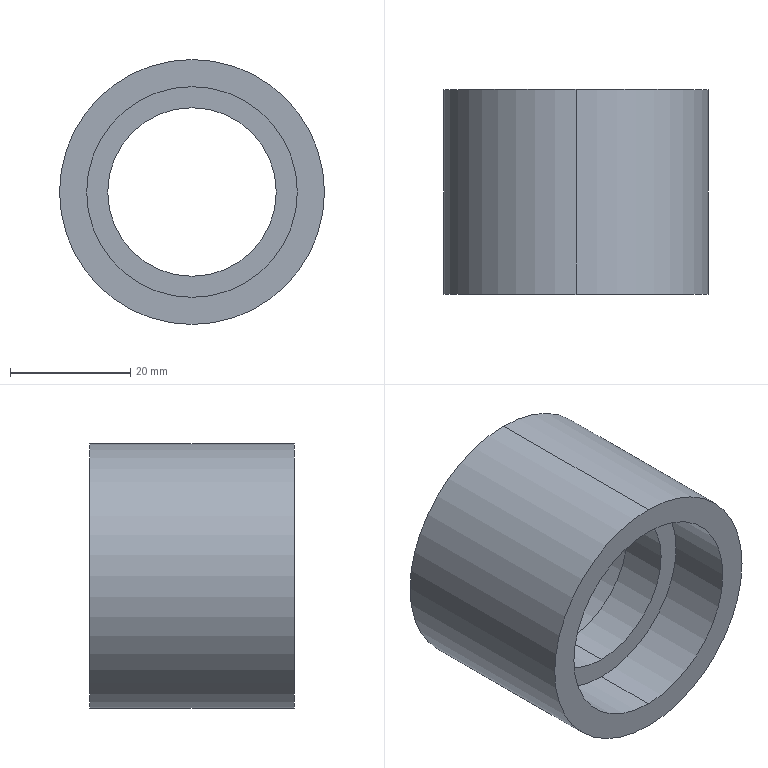Part | SolidWorks | features BaseBody 1 | 1 solid | 12 faces | box 44 x 34 x 44 mm | volume 21757 mm3 | cylinder 8 | plane 4 | commonest cylinder face diameters 35 x4 28 x2 44 x2
STEP:
#1=CARTESIAN_POINT('',(0.,17.,-22.));
#2=VERTEX_POINT('',#1);
#3=CARTESIAN_POINT('',(0.,17.,22.));
#4=VERTEX_POINT('',#3);
#5=CARTESIAN_POINT('',(0.,17.,0.));
#6=DIRECTION('',(0.,-1.,0.));
#7=DIRECTION('',(0.,0.,-1.));
#8=AXIS2_PLACEMENT_3D('',#5,#6,#7);
#9=CIRCLE('',#8,22.);
#10=EDGE_CURVE('',#2,#4,#9,.T.);
#11=ORIENTED_EDGE('',*,*,#10,.T.);
#12=CARTESIAN_POINT('',(0.,-17.,22.));
#13=VERTEX_POINT('',#12);
#14=CARTESIAN_POINT('',(0.,17.,22.));
#15=DIRECTION('',(0.,-1.,0.));
#16=VECTOR('',#15,1000.);
#17=LINE('',#14,#16);
#18=EDGE_CURVE('',#4,#13,#17,.T.);
#19=ORIENTED_EDGE('',*,*,#18,.T.);
#20=CARTESIAN_POINT('',(0.,-17.,-22.));
#21=VERTEX_POINT('',#20);
#22=CARTESIAN_POINT('',(0.,-17.,0.));
#23=DIRECTION('',(0.,1.,0.));
#24=DIRECTION('',(0.,0.,-1.));
#25=AXIS2_PLACEMENT_3D('',#22,#23,#24);
#26=CIRCLE('',#25,22.);
#27=EDGE_CURVE('',#13,#21,#26,.T.);
#28=ORIENTED_EDGE('',*,*,#27,.T.);
#29=CARTESIAN_POINT('',(0.,17.,-22.));
#30=DIRECTION('',(0.,-1.,0.));
#31=VECTOR('',#30,1000.);
#32=LINE('',#29,#31);
#33=EDGE_CURVE('',#2,#21,#32,.T.);
#34=ORIENTED_EDGE('',*,*,#33,.F.);
#35=EDGE_LOOP('',(#11,#19,#28,#34));
#36=FACE_OUTER_BOUND('',#35,.T.);
#37=CARTESIAN_POINT('',(0.,17.,0.));
#38=DIRECTION('',(0.,-1.,0.));
#39=DIRECTION('',(0.,0.,-1.));
#40=AXIS2_PLACEMENT_3D('',#37,#38,#39);
#41=CYLINDRICAL_SURFACE('',#40,22.);
#42=ADVANCED_FACE('',(#36),#41,.T.);
#43=CARTESIAN_POINT('',(0.,-6.,17.5));
#44=VERTEX_POINT('',#43);
#45=CARTESIAN_POINT('',(0.,-6.,-17.5));
#46=VERTEX_POINT('',#45);
#47=CARTESIAN_POINT('',(0.,-6.,0.));
#48=DIRECTION('',(0.,-1.,0.));
#49=DIRECTION('',(0.,0.,-1.));
#50=AXIS2_PLACEMENT_3D('',#47,#48,#49);
#51=CIRCLE('',#50,17.5);
#52=EDGE_CURVE('',#44,#46,#51,.T.);
#53=ORIENTED_EDGE('',*,*,#52,.F.);
#54=CARTESIAN_POINT('',(0.,-17.,17.5));
#55=VERTEX_POINT('',#54);
#56=CARTESIAN_POINT('',(0.,-6.,17.5));
#57=DIRECTION('',(0.,-1.,0.));
#58=VECTOR('',#57,1000.);
#59=LINE('',#56,#58);
#60=EDGE_CURVE('',#44,#55,#59,.T.);
#61=ORIENTED_EDGE('',*,*,#60,.T.);
#62=CARTESIAN_POINT('',(0.,-17.,-17.5));
#63=VERTEX_POINT('',#62);
#64=CARTESIAN_POINT('',(0.,-17.,0.));
#65=DIRECTION('',(0.,-1.,0.));
#66=DIRECTION('',(0.,0.,-1.));
#67=AXIS2_PLACEMENT_3D('',#64,#65,#66);
#68=CIRCLE('',#67,17.5);
#69=EDGE_CURVE('',#55,#63,#68,.T.);
#70=ORIENTED_EDGE('',*,*,#69,.T.);
#71=CARTESIAN_POINT('',(0.,-6.,-17.5));
#72=DIRECTION('',(0.,-1.,0.));
#73=VECTOR('',#72,1000.);
#74=LINE('',#71,#73);
#75=EDGE_CURVE('',#46,#63,#74,.T.);
#76=ORIENTED_EDGE('',*,*,#75,.F.);
#77=EDGE_LOOP('',(#53,#61,#70,#76));
#78=FACE_OUTER_BOUND('',#77,.T.);
#79=CARTESIAN_POINT('',(0.,-6.,0.));
#80=DIRECTION('',(0.,-1.,0.));
#81=DIRECTION('',(0.,0.,-1.));
#82=AXIS2_PLACEMENT_3D('',#79,#80,#81);
#83=CYLINDRICAL_SURFACE('',#82,17.5);
#84=ADVANCED_FACE('',(#78),#83,.F.);
#85=CARTESIAN_POINT('',(0.,2.,-17.5));
#86=VERTEX_POINT('',#85);
#87=CARTESIAN_POINT('',(0.,2.,17.5));
#88=VERTEX_POINT('',#87);
#89=CARTESIAN_POINT('',(0.,2.,0.));
#90=DIRECTION('',(0.,1.,0.));
#91=DIRECTION('',(0.,0.,1.));
#92=AXIS2_PLACEMENT_3D('',#89,#90,#91);
#93=CIRCLE('',#92,17.5);
#94=EDGE_CURVE('',#86,#88,#93,.T.);
#95=ORIENTED_EDGE('',*,*,#94,.F.);
#96=CARTESIAN_POINT('',(0.,17.,-17.5));
#97=VERTEX_POINT('',#96);
#98=CARTESIAN_POINT('',(0.,2.,-17.5));
#99=DIRECTION('',(0.,1.,0.));
#100=VECTOR('',#99,1000.);
#101=LINE('',#98,#100);
#102=EDGE_CURVE('',#86,#97,#101,.T.);
#103=ORIENTED_EDGE('',*,*,#102,.T.);
#104=CARTESIAN_POINT('',(0.,17.,17.5));
#105=VERTEX_POINT('',#104);
#106=CARTESIAN_POINT('',(0.,17.,0.));
#107=DIRECTION('',(0.,-1.,0.));
#108=DIRECTION('',(0.,0.,1.));
#109=AXIS2_PLACEMENT_3D('',#106,#107,#108);
#110=CIRCLE('',#109,17.5);
#111=EDGE_CURVE('',#105,#97,#110,.T.);
#112=ORIENTED_EDGE('',*,*,#111,.F.);
#113=CARTESIAN_POINT('',(0.,2.,17.5));
#114=DIRECTION('',(0.,1.,0.));
#115=VECTOR('',#114,1000.);
#116=LINE('',#113,#115);
#117=EDGE_CURVE('',#88,#105,#116,.T.);
#118=ORIENTED_EDGE('',*,*,#117,.F.);
#119=EDGE_LOOP('',(#95,#103,#112,#118));
#120=FACE_OUTER_BOUND('',#119,.T.);
#121=CARTESIAN_POINT('',(0.,2.,0.));
#122=DIRECTION('',(0.,1.,0.));
#123=DIRECTION('',(0.,0.,1.));
#124=AXIS2_PLACEMENT_3D('',#121,#122,#123);
#125=CYLINDRICAL_SURFACE('',#124,17.5);
#126=ADVANCED_FACE('',(#120),#125,.F.);
#127=CARTESIAN_POINT('',(0.,-6.,-14.));
#128=VERTEX_POINT('',#127);
#129=CARTESIAN_POINT('',(0.,-6.,14.));
#130=VERTEX_POINT('',#129);
#131=CARTESIAN_POINT('',(0.,-6.,0.));
#132=DIRECTION('',(0.,1.,0.));
#133=DIRECTION('',(0.,0.,1.));
#134=AXIS2_PLACEMENT_3D('',#131,#132,#133);
#135=CIRCLE('',#134,14.);
#136=EDGE_CURVE('',#128,#130,#135,.T.);
#137=ORIENTED_EDGE('',*,*,#136,.F.);
#138=CARTESIAN_POINT('',(0.,2.,-14.));
#139=VERTEX_POINT('',#138);
#140=CARTESIAN_POINT('',(0.,-17.,-14.));
#141=DIRECTION('',(0.,1.,0.));
#142=VECTOR('',#141,1000.);
#143=LINE('',#140,#142);
#144=EDGE_CURVE('',#128,#139,#143,.T.);
#145=ORIENTED_EDGE('',*,*,#144,.T.);
#146=CARTESIAN_POINT('',(0.,2.,14.));
#147=VERTEX_POINT('',#146);
#148=CARTESIAN_POINT('',(0.,2.,0.));
#149=DIRECTION('',(0.,-1.,0.));
#150=DIRECTION('',(0.,0.,1.));
#151=AXIS2_PLACEMENT_3D('',#148,#149,#150);
#152=CIRCLE('',#151,14.);
#153=EDGE_CURVE('',#147,#139,#152,.T.);
#154=ORIENTED_EDGE('',*,*,#153,.F.);
#155=CARTESIAN_POINT('',(0.,-17.,14.));
#156=DIRECTION('',(0.,1.,0.));
#157=VECTOR('',#156,1000.);
#158=LINE('',#155,#157);
#159=EDGE_CURVE('',#130,#147,#158,.T.);
#160=ORIENTED_EDGE('',*,*,#159,.F.);
#161=EDGE_LOOP('',(#137,#145,#154,#160));
#162=FACE_OUTER_BOUND('',#161,.T.);
#163=CARTESIAN_POINT('',(0.,-17.,0.));
#164=DIRECTION('',(0.,1.,0.));
#165=DIRECTION('',(0.,0.,1.));
#166=AXIS2_PLACEMENT_3D('',#163,#164,#165);
#167=CYLINDRICAL_SURFACE('',#166,14.);
#168=ADVANCED_FACE('',(#162),#167,.F.);
#169=ORIENTED_EDGE('',*,*,#18,.F.);
#170=CARTESIAN_POINT('',(0.,17.,0.));
#171=DIRECTION('',(0.,-1.,0.));
#172=DIRECTION('',(0.,0.,-1.));
#173=AXIS2_PLACEMENT_3D('',#170,#171,#172);
#174=CIRCLE('',#173,22.);
#175=EDGE_CURVE('',#4,#2,#174,.T.);
#176=ORIENTED_EDGE('',*,*,#175,.T.);
#177=ORIENTED_EDGE('',*,*,#33,.T.);
#178=CARTESIAN_POINT('',(0.,-17.,0.));
#179=DIRECTION('',(0.,1.,0.));
#180=DIRECTION('',(0.,0.,-1.));
#181=AXIS2_PLACEMENT_3D('',#178,#179,#180);
#182=CIRCLE('',#181,22.);
#183=EDGE_CURVE('',#21,#13,#182,.T.);
#184=ORIENTED_EDGE('',*,*,#183,.T.);
#185=EDGE_LOOP('',(#169,#176,#177,#184));
#186=FACE_OUTER_BOUND('',#185,.T.);
#187=CARTESIAN_POINT('',(0.,17.,0.));
#188=DIRECTION('',(0.,-1.,0.));
#189=DIRECTION('',(0.,0.,-1.));
#190=AXIS2_PLACEMENT_3D('',#187,#188,#189);
#191=CYLINDRICAL_SURFACE('',#190,22.);
#192=ADVANCED_FACE('',(#186),#191,.T.);
#193=ORIENTED_EDGE('',*,*,#183,.F.);
#194=ORIENTED_EDGE('',*,*,#27,.F.);
#195=EDGE_LOOP('',(#193,#194));
#196=FACE_OUTER_BOUND('',#195,.T.);
#197=CARTESIAN_POINT('',(0.,-17.,0.));
#198=DIRECTION('',(0.,-1.,0.));
#199=DIRECTION('',(0.,0.,-1.));
#200=AXIS2_PLACEMENT_3D('',#197,#198,#199);
#201=CIRCLE('',#200,17.5);
#202=EDGE_CURVE('',#63,#55,#201,.T.);
#203=ORIENTED_EDGE('',*,*,#202,.F.);
#204=ORIENTED_EDGE('',*,*,#69,.F.);
#205=EDGE_LOOP('',(#203,#204));
#206=FACE_BOUND('',#205,.T.);
#207=CARTESIAN_POINT('',(0.,-17.,0.));
#208=DIRECTION('',(0.,1.,0.));
#209=DIRECTION('',(0.,0.,1.));
#210=AXIS2_PLACEMENT_3D('',#207,#208,#209);
#211=PLANE('',#210);
#212=ADVANCED_FACE('',(#196,#206),#211,.F.);
#213=ORIENTED_EDGE('',*,*,#10,.F.);
#214=ORIENTED_EDGE('',*,*,#175,.F.);
#215=EDGE_LOOP('',(#213,#214));
#216=FACE_OUTER_BOUND('',#215,.T.);
#217=ORIENTED_EDGE('',*,*,#111,.T.);
#218=CARTESIAN_POINT('',(0.,17.,0.));
#219=DIRECTION('',(0.,-1.,0.));
#220=DIRECTION('',(0.,0.,1.));
#221=AXIS2_PLACEMENT_3D('',#218,#219,#220);
#222=CIRCLE('',#221,17.5);
#223=EDGE_CURVE('',#97,#105,#222,.T.);
#224=ORIENTED_EDGE('',*,*,#223,.T.);
#225=EDGE_LOOP('',(#217,#224));
#226=FACE_BOUND('',#225,.T.);
#227=CARTESIAN_POINT('',(0.,17.,0.));
#228=DIRECTION('',(0.,1.,0.));
#229=DIRECTION('',(0.,0.,1.));
#230=AXIS2_PLACEMENT_3D('',#227,#228,#229);
#231=PLANE('',#230);
#232=ADVANCED_FACE('',(#216,#226),#231,.T.);
#233=ORIENTED_EDGE('',*,*,#60,.F.);
#234=CARTESIAN_POINT('',(0.,-6.,0.));
#235=DIRECTION('',(0.,-1.,0.));
#236=DIRECTION('',(0.,0.,-1.));
#237=AXIS2_PLACEMENT_3D('',#234,#235,#236);
#238=CIRCLE('',#237,17.5);
#239=EDGE_CURVE('',#46,#44,#238,.T.);
#240=ORIENTED_EDGE('',*,*,#239,.F.);
#241=ORIENTED_EDGE('',*,*,#75,.T.);
#242=ORIENTED_EDGE('',*,*,#202,.T.);
#243=EDGE_LOOP('',(#233,#240,#241,#242));
#244=FACE_OUTER_BOUND('',#243,.T.);
#245=CARTESIAN_POINT('',(0.,-6.,0.));
#246=DIRECTION('',(0.,-1.,0.));
#247=DIRECTION('',(0.,0.,-1.));
#248=AXIS2_PLACEMENT_3D('',#245,#246,#247);
#249=CYLINDRICAL_SURFACE('',#248,17.5);
#250=ADVANCED_FACE('',(#244),#249,.F.);
#251=ORIENTED_EDGE('',*,*,#102,.F.);
#252=CARTESIAN_POINT('',(0.,2.,0.));
#253=DIRECTION('',(0.,1.,0.));
#254=DIRECTION('',(0.,0.,1.));
#255=AXIS2_PLACEMENT_3D('',#252,#253,#254);
#256=CIRCLE('',#255,17.5);
#257=EDGE_CURVE('',#88,#86,#256,.T.);
#258=ORIENTED_EDGE('',*,*,#257,.F.);
#259=ORIENTED_EDGE('',*,*,#117,.T.);
#260=ORIENTED_EDGE('',*,*,#223,.F.);
#261=EDGE_LOOP('',(#251,#258,#259,#260));
#262=FACE_OUTER_BOUND('',#261,.T.);
#263=CARTESIAN_POINT('',(0.,2.,0.));
#264=DIRECTION('',(0.,1.,0.));
#265=DIRECTION('',(0.,0.,1.));
#266=AXIS2_PLACEMENT_3D('',#263,#264,#265);
#267=CYLINDRICAL_SURFACE('',#266,17.5);
#268=ADVANCED_FACE('',(#262),#267,.F.);
#269=CARTESIAN_POINT('',(0.,-6.,0.));
#270=DIRECTION('',(0.,1.,0.));
#271=DIRECTION('',(0.,0.,1.));
#272=AXIS2_PLACEMENT_3D('',#269,#270,#271);
#273=CIRCLE('',#272,14.);
#274=EDGE_CURVE('',#130,#128,#273,.T.);
#275=ORIENTED_EDGE('',*,*,#274,.T.);
#276=ORIENTED_EDGE('',*,*,#136,.T.);
#277=EDGE_LOOP('',(#275,#276));
#278=FACE_BOUND('',#277,.T.);
#279=ORIENTED_EDGE('',*,*,#239,.T.);
#280=ORIENTED_EDGE('',*,*,#52,.T.);
#281=EDGE_LOOP('',(#279,#280));
#282=FACE_OUTER_BOUND('',#281,.T.);
#283=CARTESIAN_POINT('',(0.,-6.,0.));
#284=DIRECTION('',(0.,-1.,0.));
#285=DIRECTION('',(0.,0.,-1.));
#286=AXIS2_PLACEMENT_3D('',#283,#284,#285);
#287=PLANE('',#286);
#288=ADVANCED_FACE('',(#278,#282),#287,.T.);
#289=ORIENTED_EDGE('',*,*,#257,.T.);
#290=ORIENTED_EDGE('',*,*,#94,.T.);
#291=EDGE_LOOP('',(#289,#290));
#292=FACE_OUTER_BOUND('',#291,.T.);
#293=ORIENTED_EDGE('',*,*,#153,.T.);
#294=CARTESIAN_POINT('',(0.,2.,0.));
#295=DIRECTION('',(0.,-1.,0.));
#296=DIRECTION('',(0.,0.,1.));
#297=AXIS2_PLACEMENT_3D('',#294,#295,#296);
#298=CIRCLE('',#297,14.);
#299=EDGE_CURVE('',#139,#147,#298,.T.);
#300=ORIENTED_EDGE('',*,*,#299,.T.);
#301=EDGE_LOOP('',(#293,#300));
#302=FACE_BOUND('',#301,.T.);
#303=CARTESIAN_POINT('',(0.,2.,0.));
#304=DIRECTION('',(0.,1.,0.));
#305=DIRECTION('',(0.,0.,1.));
#306=AXIS2_PLACEMENT_3D('',#303,#304,#305);
#307=PLANE('',#306);
#308=ADVANCED_FACE('',(#292,#302),#307,.T.);
#309=ORIENTED_EDGE('',*,*,#144,.F.);
#310=ORIENTED_EDGE('',*,*,#274,.F.);
#311=ORIENTED_EDGE('',*,*,#159,.T.);
#312=ORIENTED_EDGE('',*,*,#299,.F.);
#313=EDGE_LOOP('',(#309,#310,#311,#312));
#314=FACE_OUTER_BOUND('',#313,.T.);
#315=CARTESIAN_POINT('',(0.,-17.,0.));
#316=DIRECTION('',(0.,1.,0.));
#317=DIRECTION('',(0.,0.,1.));
#318=AXIS2_PLACEMENT_3D('',#315,#316,#317);
#319=CYLINDRICAL_SURFACE('',#318,14.);
#320=ADVANCED_FACE('',(#314),#319,.F.);
#321=CLOSED_SHELL('',(#42,#84,#126,#168,#192,#212,#232,#250,#268,#288,#308,#320));
#322=MANIFOLD_SOLID_BREP('',#321);
#323=CARTESIAN_POINT('',(0.,0.,0.));
#324=DIRECTION('',(0.,0.,1.));
#325=DIRECTION('',(1.,0.,0.));
#326=AXIS2_PLACEMENT_3D('',#323,#324,#325);
#327=(LENGTH_UNIT()NAMED_UNIT(*)SI_UNIT(.MILLI.,.METRE.));
#328=UNCERTAINTY_MEASURE_WITH_UNIT(LENGTH_MEASURE(0.00001),#327,'','');
#329=(NAMED_UNIT(*)PLANE_ANGLE_UNIT()SI_UNIT($,.RADIAN.));
#330=(NAMED_UNIT(*)SI_UNIT($,.STERADIAN.)SOLID_ANGLE_UNIT());
#331=(GEOMETRIC_REPRESENTATION_CONTEXT(3)GLOBAL_UNCERTAINTY_ASSIGNED_CONTEXT((#328))GLOBAL_UNIT_ASSIGNED_CONTEXT((#327,#329,#330))REPRESENTATION_CONTEXT('',''));
#332=ADVANCED_BREP_SHAPE_REPRESENTATION('',(#322,#326),#331);